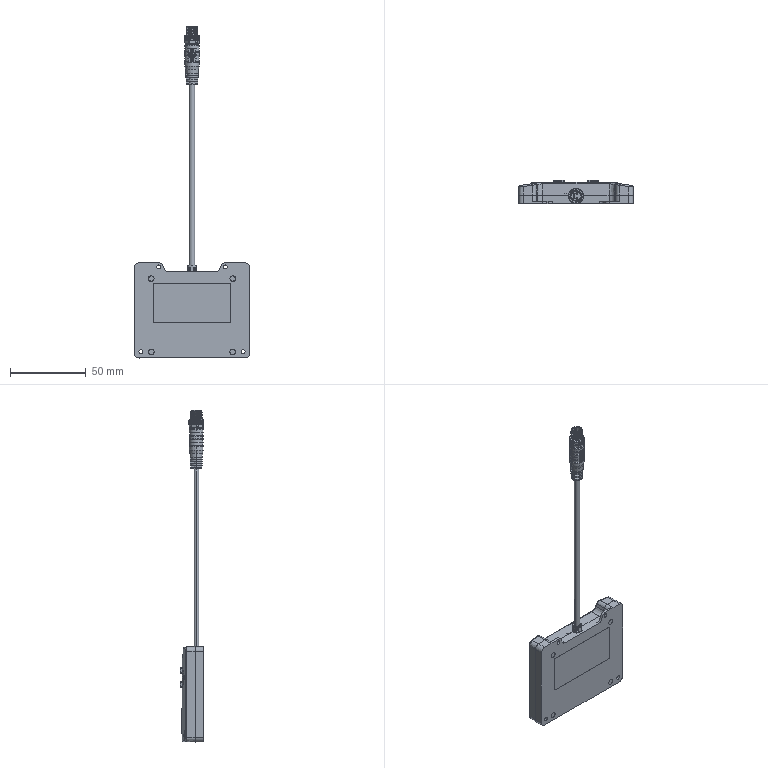Part | SolidWorks | features BaseBody 13, Revolution 2, ICE 1 | 13 solids | 2910 faces | box 76 x 15.652 x 219.462 mm | volume 48611 mm3 | plane 1400 | cylinder 983 | cone 230 | spline 185 | torus 102 | sphere 10 | commonest cylinder face diameters 0.4 x113 2 x113 1 x64 1.8 x56 0.2 x52 10 x40